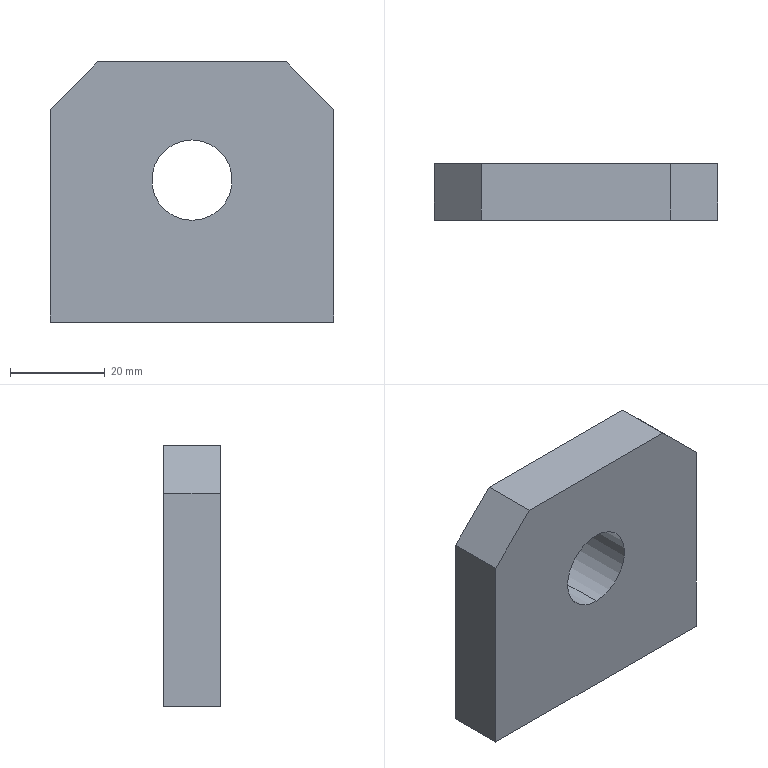Part | SolidWorks | features Chamfer 1, Extrusion 1 | 1 solid | 10 faces | box 60 x 12 x 55 mm | volume 35676 mm3 | plane 8 | cylinder 2 | commonest cylinder face diameters 17 x2
STEP:
#1=CARTESIAN_POINT('',(30.,12.,21.5));
#2=VERTEX_POINT('',#1);
#3=CARTESIAN_POINT('',(30.,12.,38.5));
#4=VERTEX_POINT('',#3);
#5=CARTESIAN_POINT('',(30.,12.,30.));
#6=DIRECTION('',(0.,1.,0.));
#7=DIRECTION('',(0.,0.,1.));
#8=AXIS2_PLACEMENT_3D('',#5,#6,#7);
#9=CIRCLE('',#8,8.5);
#10=EDGE_CURVE('',#2,#4,#9,.T.);
#11=ORIENTED_EDGE('',*,*,#10,.T.);
#12=CARTESIAN_POINT('',(30.,0.,38.5));
#13=VERTEX_POINT('',#12);
#14=CARTESIAN_POINT('',(30.,12.,38.5));
#15=DIRECTION('',(0.,-1.,0.));
#16=VECTOR('',#15,1000.);
#17=LINE('',#14,#16);
#18=EDGE_CURVE('',#4,#13,#17,.T.);
#19=ORIENTED_EDGE('',*,*,#18,.T.);
#20=CARTESIAN_POINT('',(30.,0.,21.5));
#21=VERTEX_POINT('',#20);
#22=CARTESIAN_POINT('',(30.,0.,30.));
#23=DIRECTION('',(0.,1.,0.));
#24=DIRECTION('',(0.,0.,1.));
#25=AXIS2_PLACEMENT_3D('',#22,#23,#24);
#26=CIRCLE('',#25,8.5);
#27=EDGE_CURVE('',#21,#13,#26,.T.);
#28=ORIENTED_EDGE('',*,*,#27,.F.);
#29=CARTESIAN_POINT('',(30.,12.,21.5));
#30=DIRECTION('',(0.,-1.,0.));
#31=VECTOR('',#30,1000.);
#32=LINE('',#29,#31);
#33=EDGE_CURVE('',#2,#21,#32,.T.);
#34=ORIENTED_EDGE('',*,*,#33,.F.);
#35=EDGE_LOOP('',(#11,#19,#28,#34));
#36=FACE_OUTER_BOUND('',#35,.T.);
#37=CARTESIAN_POINT('',(30.,12.,30.));
#38=DIRECTION('',(0.,-1.,0.));
#39=DIRECTION('',(0.,0.,-1.));
#40=AXIS2_PLACEMENT_3D('',#37,#38,#39);
#41=CYLINDRICAL_SURFACE('',#40,8.5);
#42=ADVANCED_FACE('',(#36),#41,.F.);
#43=CARTESIAN_POINT('',(10.,12.,55.));
#44=VERTEX_POINT('',#43);
#45=CARTESIAN_POINT('',(50.,12.,55.));
#46=VERTEX_POINT('',#45);
#47=CARTESIAN_POINT('',(0.,12.,55.));
#48=DIRECTION('',(1.,0.,0.));
#49=VECTOR('',#48,1000.);
#50=LINE('',#47,#49);
#51=EDGE_CURVE('',#44,#46,#50,.T.);
#52=ORIENTED_EDGE('',*,*,#51,.T.);
#53=CARTESIAN_POINT('',(60.,12.,45.));
#54=VERTEX_POINT('',#53);
#55=CARTESIAN_POINT('',(52.5,12.,52.5));
#56=DIRECTION('',(0.7071,0.,-0.7071));
#57=VECTOR('',#56,1000.);
#58=LINE('',#55,#57);
#59=EDGE_CURVE('',#46,#54,#58,.T.);
#60=ORIENTED_EDGE('',*,*,#59,.T.);
#61=CARTESIAN_POINT('',(60.,12.,0.));
#62=VERTEX_POINT('',#61);
#63=CARTESIAN_POINT('',(60.,12.,0.));
#64=DIRECTION('',(0.,0.,-1.));
#65=VECTOR('',#64,1000.);
#66=LINE('',#63,#65);
#67=EDGE_CURVE('',#54,#62,#66,.T.);
#68=ORIENTED_EDGE('',*,*,#67,.T.);
#69=CARTESIAN_POINT('',(0.,12.,0.));
#70=VERTEX_POINT('',#69);
#71=CARTESIAN_POINT('',(0.,12.,0.));
#72=DIRECTION('',(-1.,0.,0.));
#73=VECTOR('',#72,1000.);
#74=LINE('',#71,#73);
#75=EDGE_CURVE('',#62,#70,#74,.T.);
#76=ORIENTED_EDGE('',*,*,#75,.T.);
#77=CARTESIAN_POINT('',(0.,12.,45.));
#78=VERTEX_POINT('',#77);
#79=CARTESIAN_POINT('',(0.,12.,0.));
#80=DIRECTION('',(0.,0.,1.));
#81=VECTOR('',#80,1000.);
#82=LINE('',#79,#81);
#83=EDGE_CURVE('',#70,#78,#82,.T.);
#84=ORIENTED_EDGE('',*,*,#83,.T.);
#85=CARTESIAN_POINT('',(-22.5,12.,22.5));
#86=DIRECTION('',(0.7071,0.,0.7071));
#87=VECTOR('',#86,1000.);
#88=LINE('',#85,#87);
#89=EDGE_CURVE('',#78,#44,#88,.T.);
#90=ORIENTED_EDGE('',*,*,#89,.T.);
#91=EDGE_LOOP('',(#52,#60,#68,#76,#84,#90));
#92=FACE_OUTER_BOUND('',#91,.T.);
#93=ORIENTED_EDGE('',*,*,#10,.F.);
#94=CARTESIAN_POINT('',(30.,12.,30.));
#95=DIRECTION('',(0.,1.,0.));
#96=DIRECTION('',(0.,0.,1.));
#97=AXIS2_PLACEMENT_3D('',#94,#95,#96);
#98=CIRCLE('',#97,8.5);
#99=EDGE_CURVE('',#4,#2,#98,.T.);
#100=ORIENTED_EDGE('',*,*,#99,.F.);
#101=EDGE_LOOP('',(#93,#100));
#102=FACE_BOUND('',#101,.T.);
#103=CARTESIAN_POINT('',(0.,12.,0.));
#104=DIRECTION('',(0.,1.,0.));
#105=DIRECTION('',(0.,0.,1.));
#106=AXIS2_PLACEMENT_3D('',#103,#104,#105);
#107=PLANE('',#106);
#108=ADVANCED_FACE('',(#92,#102),#107,.T.);
#109=CARTESIAN_POINT('',(60.,0.,45.));
#110=VERTEX_POINT('',#109);
#111=CARTESIAN_POINT('',(60.,0.,0.));
#112=VERTEX_POINT('',#111);
#113=CARTESIAN_POINT('',(60.,0.,0.));
#114=DIRECTION('',(0.,0.,-1.));
#115=VECTOR('',#114,1000.);
#116=LINE('',#113,#115);
#117=EDGE_CURVE('',#110,#112,#116,.T.);
#118=ORIENTED_EDGE('',*,*,#117,.F.);
#119=CARTESIAN_POINT('',(50.,0.,55.));
#120=VERTEX_POINT('',#119);
#121=CARTESIAN_POINT('',(60.,0.,45.));
#122=DIRECTION('',(-0.7071,0.,0.7071));
#123=VECTOR('',#122,1000.);
#124=LINE('',#121,#123);
#125=EDGE_CURVE('',#110,#120,#124,.T.);
#126=ORIENTED_EDGE('',*,*,#125,.T.);
#127=CARTESIAN_POINT('',(10.,0.,55.));
#128=VERTEX_POINT('',#127);
#129=CARTESIAN_POINT('',(0.,0.,55.));
#130=DIRECTION('',(1.,0.,0.));
#131=VECTOR('',#130,1000.);
#132=LINE('',#129,#131);
#133=EDGE_CURVE('',#128,#120,#132,.T.);
#134=ORIENTED_EDGE('',*,*,#133,.F.);
#135=CARTESIAN_POINT('',(0.,0.,45.));
#136=VERTEX_POINT('',#135);
#137=CARTESIAN_POINT('',(10.,0.,55.));
#138=DIRECTION('',(-0.7071,0.,-0.7071));
#139=VECTOR('',#138,1000.);
#140=LINE('',#137,#139);
#141=EDGE_CURVE('',#128,#136,#140,.T.);
#142=ORIENTED_EDGE('',*,*,#141,.T.);
#143=CARTESIAN_POINT('',(0.,0.,0.));
#144=VERTEX_POINT('',#143);
#145=CARTESIAN_POINT('',(0.,0.,0.));
#146=DIRECTION('',(0.,0.,1.));
#147=VECTOR('',#146,1000.);
#148=LINE('',#145,#147);
#149=EDGE_CURVE('',#144,#136,#148,.T.);
#150=ORIENTED_EDGE('',*,*,#149,.F.);
#151=CARTESIAN_POINT('',(0.,0.,0.));
#152=DIRECTION('',(-1.,0.,0.));
#153=VECTOR('',#152,1000.);
#154=LINE('',#151,#153);
#155=EDGE_CURVE('',#112,#144,#154,.T.);
#156=ORIENTED_EDGE('',*,*,#155,.F.);
#157=EDGE_LOOP('',(#118,#126,#134,#142,#150,#156));
#158=FACE_OUTER_BOUND('',#157,.T.);
#159=ORIENTED_EDGE('',*,*,#27,.T.);
#160=CARTESIAN_POINT('',(30.,0.,30.));
#161=DIRECTION('',(0.,1.,0.));
#162=DIRECTION('',(0.,0.,1.));
#163=AXIS2_PLACEMENT_3D('',#160,#161,#162);
#164=CIRCLE('',#163,8.5);
#165=EDGE_CURVE('',#13,#21,#164,.T.);
#166=ORIENTED_EDGE('',*,*,#165,.T.);
#167=EDGE_LOOP('',(#159,#166));
#168=FACE_BOUND('',#167,.T.);
#169=CARTESIAN_POINT('',(0.,0.,0.));
#170=DIRECTION('',(0.,1.,0.));
#171=DIRECTION('',(0.,0.,1.));
#172=AXIS2_PLACEMENT_3D('',#169,#170,#171);
#173=PLANE('',#172);
#174=ADVANCED_FACE('',(#158,#168),#173,.F.);
#175=ORIENTED_EDGE('',*,*,#149,.T.);
#176=CARTESIAN_POINT('',(0.,12.,45.));
#177=DIRECTION('',(0.,1.,0.));
#178=VECTOR('',#177,1000.);
#179=LINE('',#176,#178);
#180=EDGE_CURVE('',#136,#78,#179,.T.);
#181=ORIENTED_EDGE('',*,*,#180,.T.);
#182=ORIENTED_EDGE('',*,*,#83,.F.);
#183=CARTESIAN_POINT('',(0.,12.,0.));
#184=DIRECTION('',(0.,-1.,0.));
#185=VECTOR('',#184,1000.);
#186=LINE('',#183,#185);
#187=EDGE_CURVE('',#70,#144,#186,.T.);
#188=ORIENTED_EDGE('',*,*,#187,.T.);
#189=EDGE_LOOP('',(#175,#181,#182,#188));
#190=FACE_OUTER_BOUND('',#189,.T.);
#191=CARTESIAN_POINT('',(0.,12.,0.));
#192=DIRECTION('',(1.,0.,0.));
#193=DIRECTION('',(0.,0.,-1.));
#194=AXIS2_PLACEMENT_3D('',#191,#192,#193);
#195=PLANE('',#194);
#196=ADVANCED_FACE('',(#190),#195,.F.);
#197=ORIENTED_EDGE('',*,*,#133,.T.);
#198=CARTESIAN_POINT('',(50.,12.,55.));
#199=DIRECTION('',(0.,1.,0.));
#200=VECTOR('',#199,1000.);
#201=LINE('',#198,#200);
#202=EDGE_CURVE('',#120,#46,#201,.T.);
#203=ORIENTED_EDGE('',*,*,#202,.T.);
#204=ORIENTED_EDGE('',*,*,#51,.F.);
#205=CARTESIAN_POINT('',(10.,12.,55.));
#206=DIRECTION('',(0.,-1.,0.));
#207=VECTOR('',#206,1000.);
#208=LINE('',#205,#207);
#209=EDGE_CURVE('',#44,#128,#208,.T.);
#210=ORIENTED_EDGE('',*,*,#209,.T.);
#211=EDGE_LOOP('',(#197,#203,#204,#210));
#212=FACE_OUTER_BOUND('',#211,.T.);
#213=CARTESIAN_POINT('',(0.,12.,55.));
#214=DIRECTION('',(0.,0.,-1.));
#215=DIRECTION('',(-1.,0.,0.));
#216=AXIS2_PLACEMENT_3D('',#213,#214,#215);
#217=PLANE('',#216);
#218=ADVANCED_FACE('',(#212),#217,.F.);
#219=ORIENTED_EDGE('',*,*,#67,.F.);
#220=CARTESIAN_POINT('',(60.,12.,45.));
#221=DIRECTION('',(0.,-1.,0.));
#222=VECTOR('',#221,1000.);
#223=LINE('',#220,#222);
#224=EDGE_CURVE('',#54,#110,#223,.T.);
#225=ORIENTED_EDGE('',*,*,#224,.T.);
#226=ORIENTED_EDGE('',*,*,#117,.T.);
#227=CARTESIAN_POINT('',(60.,12.,0.));
#228=DIRECTION('',(0.,-1.,0.));
#229=VECTOR('',#228,1000.);
#230=LINE('',#227,#229);
#231=EDGE_CURVE('',#62,#112,#230,.T.);
#232=ORIENTED_EDGE('',*,*,#231,.F.);
#233=EDGE_LOOP('',(#219,#225,#226,#232));
#234=FACE_OUTER_BOUND('',#233,.T.);
#235=CARTESIAN_POINT('',(60.,12.,0.));
#236=DIRECTION('',(-1.,0.,0.));
#237=DIRECTION('',(0.,0.,1.));
#238=AXIS2_PLACEMENT_3D('',#235,#236,#237);
#239=PLANE('',#238);
#240=ADVANCED_FACE('',(#234),#239,.F.);
#241=ORIENTED_EDGE('',*,*,#155,.T.);
#242=ORIENTED_EDGE('',*,*,#187,.F.);
#243=ORIENTED_EDGE('',*,*,#75,.F.);
#244=ORIENTED_EDGE('',*,*,#231,.T.);
#245=EDGE_LOOP('',(#241,#242,#243,#244));
#246=FACE_OUTER_BOUND('',#245,.T.);
#247=CARTESIAN_POINT('',(0.,12.,0.));
#248=DIRECTION('',(0.,0.,1.));
#249=DIRECTION('',(1.,0.,0.));
#250=AXIS2_PLACEMENT_3D('',#247,#248,#249);
#251=PLANE('',#250);
#252=ADVANCED_FACE('',(#246),#251,.F.);
#253=ORIENTED_EDGE('',*,*,#18,.F.);
#254=ORIENTED_EDGE('',*,*,#99,.T.);
#255=ORIENTED_EDGE('',*,*,#33,.T.);
#256=ORIENTED_EDGE('',*,*,#165,.F.);
#257=EDGE_LOOP('',(#253,#254,#255,#256));
#258=FACE_OUTER_BOUND('',#257,.T.);
#259=CARTESIAN_POINT('',(30.,12.,30.));
#260=DIRECTION('',(0.,-1.,0.));
#261=DIRECTION('',(0.,0.,-1.));
#262=AXIS2_PLACEMENT_3D('',#259,#260,#261);
#263=CYLINDRICAL_SURFACE('',#262,8.5);
#264=ADVANCED_FACE('',(#258),#263,.F.);
#265=ORIENTED_EDGE('',*,*,#59,.F.);
#266=ORIENTED_EDGE('',*,*,#202,.F.);
#267=ORIENTED_EDGE('',*,*,#125,.F.);
#268=ORIENTED_EDGE('',*,*,#224,.F.);
#269=EDGE_LOOP('',(#265,#266,#267,#268));
#270=FACE_OUTER_BOUND('',#269,.T.);
#271=CARTESIAN_POINT('',(60.,12.,45.));
#272=DIRECTION('',(-0.7071,0.,-0.7071));
#273=DIRECTION('',(0.,-1.,0.));
#274=AXIS2_PLACEMENT_3D('',#271,#272,#273);
#275=PLANE('',#274);
#276=ADVANCED_FACE('',(#270),#275,.F.);
#277=ORIENTED_EDGE('',*,*,#89,.F.);
#278=ORIENTED_EDGE('',*,*,#180,.F.);
#279=ORIENTED_EDGE('',*,*,#141,.F.);
#280=ORIENTED_EDGE('',*,*,#209,.F.);
#281=EDGE_LOOP('',(#277,#278,#279,#280));
#282=FACE_OUTER_BOUND('',#281,.T.);
#283=CARTESIAN_POINT('',(10.,12.,55.));
#284=DIRECTION('',(0.7071,0.,-0.7071));
#285=DIRECTION('',(0.,-1.,0.));
#286=AXIS2_PLACEMENT_3D('',#283,#284,#285);
#287=PLANE('',#286);
#288=ADVANCED_FACE('',(#282),#287,.F.);
#289=CLOSED_SHELL('',(#42,#108,#174,#196,#218,#240,#252,#264,#276,#288));
#290=MANIFOLD_SOLID_BREP('',#289);
#291=CARTESIAN_POINT('',(0.,0.,0.));
#292=DIRECTION('',(0.,0.,1.));
#293=DIRECTION('',(1.,0.,0.));
#294=AXIS2_PLACEMENT_3D('',#291,#292,#293);
#295=(LENGTH_UNIT()NAMED_UNIT(*)SI_UNIT(.MILLI.,.METRE.));
#296=UNCERTAINTY_MEASURE_WITH_UNIT(LENGTH_MEASURE(0.00001),#295,'','');
#297=(NAMED_UNIT(*)PLANE_ANGLE_UNIT()SI_UNIT($,.RADIAN.));
#298=(NAMED_UNIT(*)SI_UNIT($,.STERADIAN.)SOLID_ANGLE_UNIT());
#299=(GEOMETRIC_REPRESENTATION_CONTEXT(3)GLOBAL_UNCERTAINTY_ASSIGNED_CONTEXT((#296))GLOBAL_UNIT_ASSIGNED_CONTEXT((#295,#297,#298))REPRESENTATION_CONTEXT('',''));
#300=ADVANCED_BREP_SHAPE_REPRESENTATION('',(#290,#294),#299);